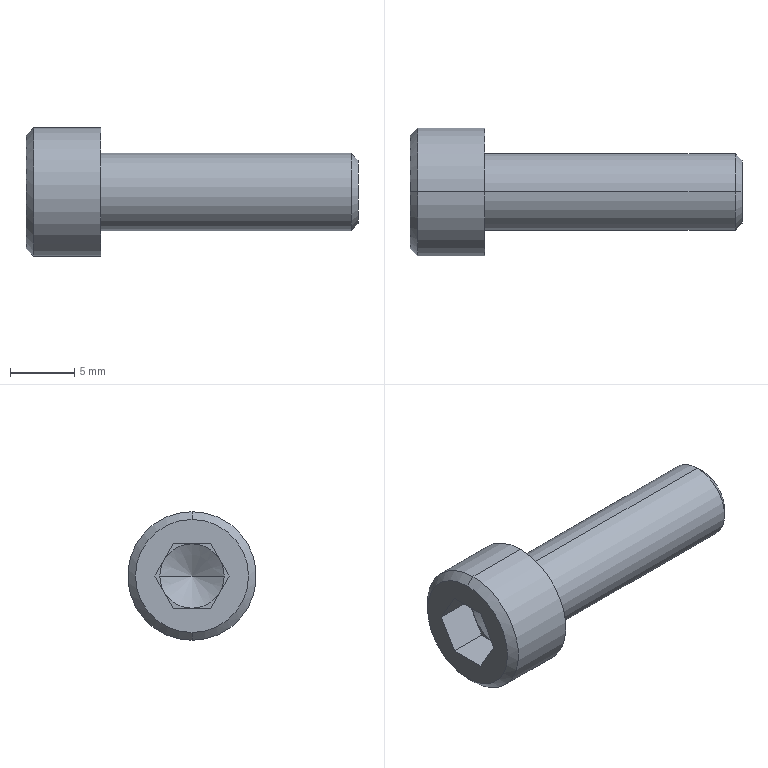Part | STEP file | 0244_Z_007_CPSWC65-16-20_2 | 1 solid | 25 faces | box 25.82 x 10 x 10 mm | volume 940.164 mm3 | plane 15 | cone 6 | cylinder 4 | commonest cylinder face diameters 6 x2 10 x2